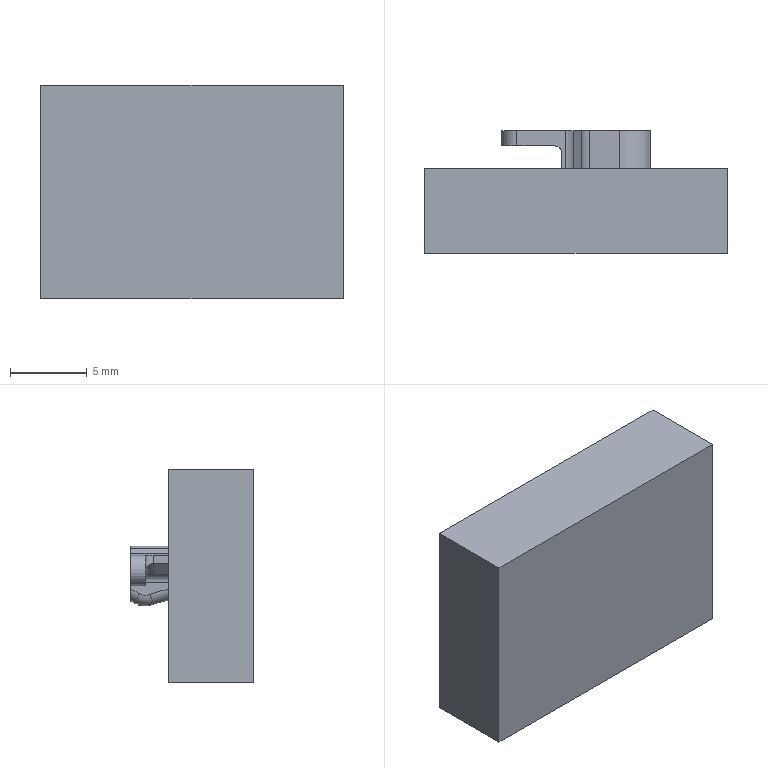Part | 2 solids | 56 faces | box 19.7 x 8 x 13.91 mm | volume 1522 mm3 | plane 28 | cylinder 25 | torus 3 | commonest cylinder face diameters 1 x10 2 x7 10 x3 1.4 x2 4 x2 1.402 x1